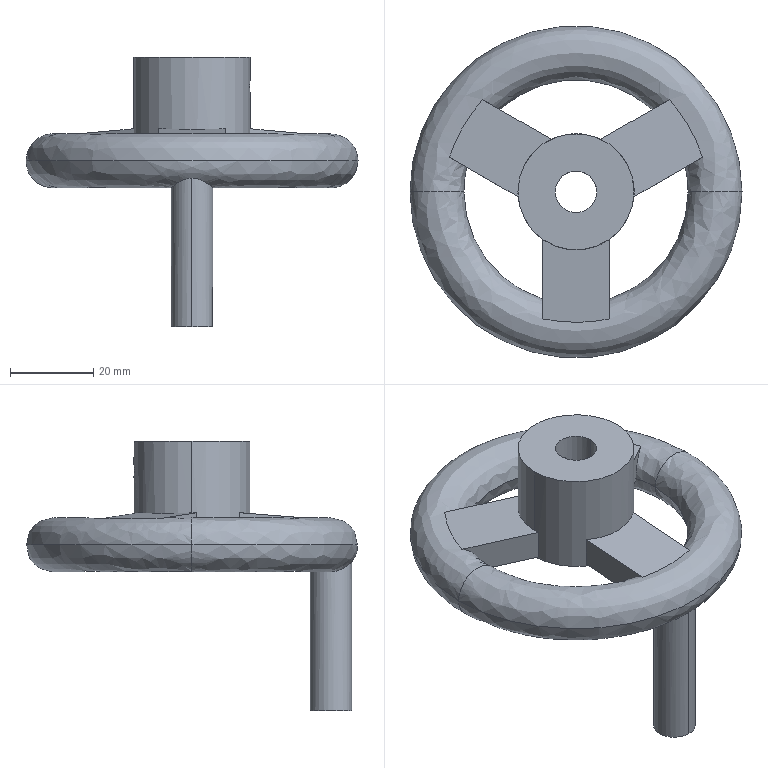Part | STEP file | Handwheel | 1 solid | 29 faces | box 80 x 80 x 65 mm | volume 48947 mm3 | plane 15 | cylinder 10 | spline 4 | commonest cylinder face diameters 3.3 x4 10 x4 28 x2